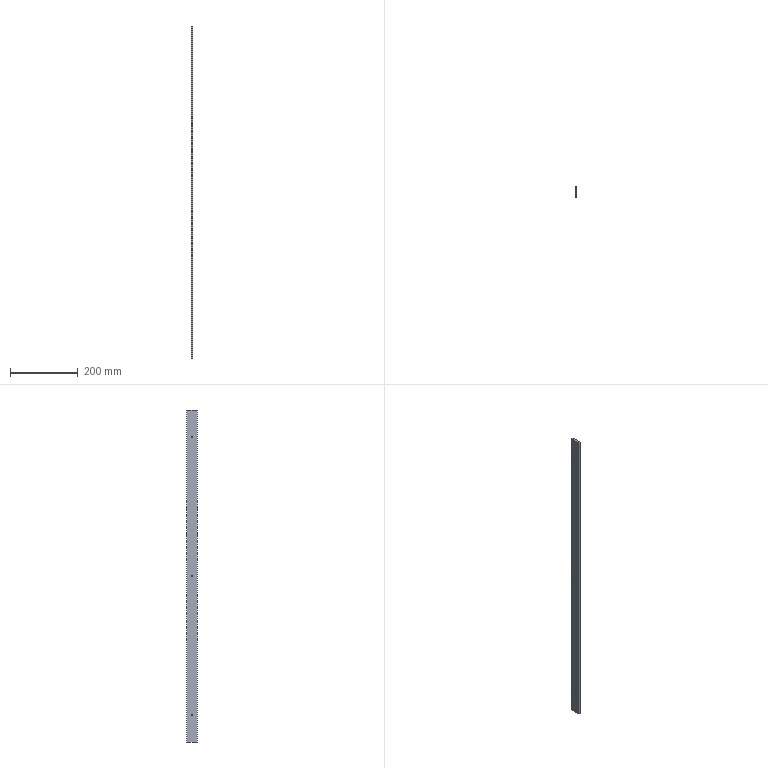Part | NX | features solid 2 | 1 solid | 12 faces | box 5 x 30 x 980 mm | volume 146715 mm3 | cylinder 6 | plane 6 | commonest cylinder face diameters 4.917 x6
STEP:
#1=CARTESIAN_POINT('',(-325.,487.459,347.));
#2=VERTEX_POINT('',#1);
#3=CARTESIAN_POINT('',(-330.,487.459,347.));
#4=VERTEX_POINT('',#3);
#5=CARTESIAN_POINT('',(650.472,487.459,347.));
#6=DIRECTION('',(-1.,0.,0.));
#7=VECTOR('',#6,1000.);
#8=LINE('',#5,#7);
#9=EDGE_CURVE('',#2,#4,#8,.T.);
#10=ORIENTED_EDGE('',*,*,#9,.F.);
#11=CARTESIAN_POINT('',(-325.,482.541,347.));
#12=VERTEX_POINT('',#11);
#13=CARTESIAN_POINT('',(-325.,485.,347.));
#14=DIRECTION('',(1.,0.,0.));
#15=DIRECTION('',(0.,1.,0.));
#16=AXIS2_PLACEMENT_3D('',#13,#14,#15);
#17=CIRCLE('',#16,2.458);
#18=EDGE_CURVE('',#2,#12,#17,.T.);
#19=ORIENTED_EDGE('',*,*,#18,.T.);
#20=CARTESIAN_POINT('',(-330.,482.541,347.));
#21=VERTEX_POINT('',#20);
#22=CARTESIAN_POINT('',(650.472,482.541,347.));
#23=DIRECTION('',(-1.,0.,0.));
#24=VECTOR('',#23,1000.);
#25=LINE('',#22,#24);
#26=EDGE_CURVE('',#21,#12,#25,.F.);
#27=ORIENTED_EDGE('',*,*,#26,.F.);
#28=CARTESIAN_POINT('',(-330.,485.,347.));
#29=DIRECTION('',(-1.,0.,0.));
#30=DIRECTION('',(0.,0.,1.));
#31=AXIS2_PLACEMENT_3D('',#28,#29,#30);
#32=CIRCLE('',#31,2.458);
#33=EDGE_CURVE('',#21,#4,#32,.T.);
#34=ORIENTED_EDGE('',*,*,#33,.T.);
#35=EDGE_LOOP('',(#10,#19,#27,#34));
#36=FACE_BOUND('',#35,.T.);
#37=CARTESIAN_POINT('',(650.472,485.,347.));
#38=DIRECTION('',(-1.,0.,0.));
#39=DIRECTION('',(0.,-1.,0.));
#40=AXIS2_PLACEMENT_3D('',#37,#38,#39);
#41=CYLINDRICAL_SURFACE('',#40,2.458);
#42=ADVANCED_FACE('',(#36),#41,.F.);
#43=CARTESIAN_POINT('',(-325.,487.459,1167.));
#44=VERTEX_POINT('',#43);
#45=CARTESIAN_POINT('',(-330.,487.459,1167.));
#46=VERTEX_POINT('',#45);
#47=CARTESIAN_POINT('',(650.472,487.459,1167.));
#48=DIRECTION('',(-1.,0.,0.));
#49=VECTOR('',#48,1000.);
#50=LINE('',#47,#49);
#51=EDGE_CURVE('',#44,#46,#50,.T.);
#52=ORIENTED_EDGE('',*,*,#51,.F.);
#53=CARTESIAN_POINT('',(-325.,482.541,1167.));
#54=VERTEX_POINT('',#53);
#55=CARTESIAN_POINT('',(-325.,485.,1167.));
#56=DIRECTION('',(1.,0.,0.));
#57=DIRECTION('',(0.,1.,0.));
#58=AXIS2_PLACEMENT_3D('',#55,#56,#57);
#59=CIRCLE('',#58,2.458);
#60=EDGE_CURVE('',#44,#54,#59,.T.);
#61=ORIENTED_EDGE('',*,*,#60,.T.);
#62=CARTESIAN_POINT('',(-330.,482.541,1167.));
#63=VERTEX_POINT('',#62);
#64=CARTESIAN_POINT('',(650.472,482.541,1167.));
#65=DIRECTION('',(-1.,0.,0.));
#66=VECTOR('',#65,1000.);
#67=LINE('',#64,#66);
#68=EDGE_CURVE('',#63,#54,#67,.F.);
#69=ORIENTED_EDGE('',*,*,#68,.F.);
#70=CARTESIAN_POINT('',(-330.,485.,1167.));
#71=DIRECTION('',(-1.,0.,0.));
#72=DIRECTION('',(0.,0.,1.));
#73=AXIS2_PLACEMENT_3D('',#70,#71,#72);
#74=CIRCLE('',#73,2.458);
#75=EDGE_CURVE('',#63,#46,#74,.T.);
#76=ORIENTED_EDGE('',*,*,#75,.T.);
#77=EDGE_LOOP('',(#52,#61,#69,#76));
#78=FACE_BOUND('',#77,.T.);
#79=CARTESIAN_POINT('',(650.472,485.,1167.));
#80=DIRECTION('',(-1.,0.,0.));
#81=DIRECTION('',(0.,-1.,0.));
#82=AXIS2_PLACEMENT_3D('',#79,#80,#81);
#83=CYLINDRICAL_SURFACE('',#82,2.458);
#84=ADVANCED_FACE('',(#78),#83,.F.);
#85=CARTESIAN_POINT('',(-330.,487.459,757.));
#86=VERTEX_POINT('',#85);
#87=CARTESIAN_POINT('',(-325.,487.459,757.));
#88=VERTEX_POINT('',#87);
#89=CARTESIAN_POINT('',(650.472,487.459,757.));
#90=DIRECTION('',(-1.,0.,0.));
#91=VECTOR('',#90,1000.);
#92=LINE('',#89,#91);
#93=EDGE_CURVE('',#86,#88,#92,.F.);
#94=ORIENTED_EDGE('',*,*,#93,.T.);
#95=CARTESIAN_POINT('',(-325.,482.541,757.));
#96=VERTEX_POINT('',#95);
#97=CARTESIAN_POINT('',(-325.,485.,757.));
#98=DIRECTION('',(1.,0.,0.));
#99=DIRECTION('',(0.,1.,0.));
#100=AXIS2_PLACEMENT_3D('',#97,#98,#99);
#101=CIRCLE('',#100,2.458);
#102=EDGE_CURVE('',#88,#96,#101,.T.);
#103=ORIENTED_EDGE('',*,*,#102,.T.);
#104=CARTESIAN_POINT('',(-330.,482.541,757.));
#105=VERTEX_POINT('',#104);
#106=CARTESIAN_POINT('',(650.472,482.541,757.));
#107=DIRECTION('',(-1.,0.,0.));
#108=VECTOR('',#107,1000.);
#109=LINE('',#106,#108);
#110=EDGE_CURVE('',#96,#105,#109,.T.);
#111=ORIENTED_EDGE('',*,*,#110,.T.);
#112=CARTESIAN_POINT('',(-330.,485.,757.));
#113=DIRECTION('',(-1.,0.,0.));
#114=DIRECTION('',(0.,0.,1.));
#115=AXIS2_PLACEMENT_3D('',#112,#113,#114);
#116=CIRCLE('',#115,2.459);
#117=EDGE_CURVE('',#105,#86,#116,.T.);
#118=ORIENTED_EDGE('',*,*,#117,.T.);
#119=EDGE_LOOP('',(#94,#103,#111,#118));
#120=FACE_BOUND('',#119,.T.);
#121=CARTESIAN_POINT('',(650.472,485.,757.));
#122=DIRECTION('',(-1.,0.,0.));
#123=DIRECTION('',(0.,-1.,0.));
#124=AXIS2_PLACEMENT_3D('',#121,#122,#123);
#125=CYLINDRICAL_SURFACE('',#124,2.458);
#126=ADVANCED_FACE('',(#120),#125,.F.);
#127=ORIENTED_EDGE('',*,*,#117,.F.);
#128=CARTESIAN_POINT('',(-330.,485.,757.));
#129=DIRECTION('',(-1.,0.,0.));
#130=DIRECTION('',(0.,0.,1.));
#131=AXIS2_PLACEMENT_3D('',#128,#129,#130);
#132=CIRCLE('',#131,2.459);
#133=EDGE_CURVE('',#86,#105,#132,.T.);
#134=ORIENTED_EDGE('',*,*,#133,.F.);
#135=EDGE_LOOP('',(#127,#134));
#136=FACE_BOUND('',#135,.T.);
#137=ORIENTED_EDGE('',*,*,#75,.F.);
#138=CARTESIAN_POINT('',(-330.,485.,1167.));
#139=DIRECTION('',(-1.,0.,0.));
#140=DIRECTION('',(0.,0.,1.));
#141=AXIS2_PLACEMENT_3D('',#138,#139,#140);
#142=CIRCLE('',#141,2.458);
#143=EDGE_CURVE('',#46,#63,#142,.T.);
#144=ORIENTED_EDGE('',*,*,#143,.F.);
#145=EDGE_LOOP('',(#137,#144));
#146=FACE_BOUND('',#145,.T.);
#147=ORIENTED_EDGE('',*,*,#33,.F.);
#148=CARTESIAN_POINT('',(-330.,485.,347.));
#149=DIRECTION('',(-1.,0.,0.));
#150=DIRECTION('',(0.,0.,1.));
#151=AXIS2_PLACEMENT_3D('',#148,#149,#150);
#152=CIRCLE('',#151,2.458);
#153=EDGE_CURVE('',#4,#21,#152,.T.);
#154=ORIENTED_EDGE('',*,*,#153,.F.);
#155=EDGE_LOOP('',(#147,#154));
#156=FACE_BOUND('',#155,.T.);
#157=CARTESIAN_POINT('',(-330.,470.,267.));
#158=VERTEX_POINT('',#157);
#159=CARTESIAN_POINT('',(-330.,500.,267.));
#160=VERTEX_POINT('',#159);
#161=CARTESIAN_POINT('',(-330.,470.,267.));
#162=DIRECTION('',(0.,1.,0.));
#163=VECTOR('',#162,1000.);
#164=LINE('',#161,#163);
#165=EDGE_CURVE('',#158,#160,#164,.T.);
#166=ORIENTED_EDGE('',*,*,#165,.F.);
#167=CARTESIAN_POINT('',(-330.,470.,1247.));
#168=VERTEX_POINT('',#167);
#169=CARTESIAN_POINT('',(-330.,470.,1247.));
#170=DIRECTION('',(0.,0.,-1.));
#171=VECTOR('',#170,1000.);
#172=LINE('',#169,#171);
#173=EDGE_CURVE('',#168,#158,#172,.T.);
#174=ORIENTED_EDGE('',*,*,#173,.F.);
#175=CARTESIAN_POINT('',(-330.,500.,1247.));
#176=VERTEX_POINT('',#175);
#177=CARTESIAN_POINT('',(-330.,500.,1247.));
#178=DIRECTION('',(0.,-1.,0.));
#179=VECTOR('',#178,1000.);
#180=LINE('',#177,#179);
#181=EDGE_CURVE('',#176,#168,#180,.T.);
#182=ORIENTED_EDGE('',*,*,#181,.F.);
#183=CARTESIAN_POINT('',(-330.,500.,267.));
#184=DIRECTION('',(0.,0.,1.));
#185=VECTOR('',#184,1000.);
#186=LINE('',#183,#185);
#187=EDGE_CURVE('',#160,#176,#186,.T.);
#188=ORIENTED_EDGE('',*,*,#187,.F.);
#189=EDGE_LOOP('',(#166,#174,#182,#188));
#190=FACE_BOUND('',#189,.T.);
#191=CARTESIAN_POINT('',(-330.,485.,757.));
#192=DIRECTION('',(1.,0.,0.));
#193=DIRECTION('',(0.,1.,0.));
#194=AXIS2_PLACEMENT_3D('',#191,#192,#193);
#195=PLANE('',#194);
#196=ADVANCED_FACE('',(#136,#146,#156,#190),#195,.F.);
#197=CARTESIAN_POINT('',(-325.,485.,757.));
#198=DIRECTION('',(1.,0.,0.));
#199=DIRECTION('',(0.,1.,0.));
#200=AXIS2_PLACEMENT_3D('',#197,#198,#199);
#201=CIRCLE('',#200,2.458);
#202=EDGE_CURVE('',#96,#88,#201,.T.);
#203=ORIENTED_EDGE('',*,*,#202,.F.);
#204=ORIENTED_EDGE('',*,*,#102,.F.);
#205=EDGE_LOOP('',(#203,#204));
#206=FACE_BOUND('',#205,.T.);
#207=CARTESIAN_POINT('',(-325.,485.,1167.));
#208=DIRECTION('',(1.,0.,0.));
#209=DIRECTION('',(0.,1.,0.));
#210=AXIS2_PLACEMENT_3D('',#207,#208,#209);
#211=CIRCLE('',#210,2.458);
#212=EDGE_CURVE('',#54,#44,#211,.T.);
#213=ORIENTED_EDGE('',*,*,#212,.F.);
#214=ORIENTED_EDGE('',*,*,#60,.F.);
#215=EDGE_LOOP('',(#213,#214));
#216=FACE_BOUND('',#215,.T.);
#217=CARTESIAN_POINT('',(-325.,485.,347.));
#218=DIRECTION('',(1.,0.,0.));
#219=DIRECTION('',(0.,1.,0.));
#220=AXIS2_PLACEMENT_3D('',#217,#218,#219);
#221=CIRCLE('',#220,2.458);
#222=EDGE_CURVE('',#12,#2,#221,.T.);
#223=ORIENTED_EDGE('',*,*,#222,.F.);
#224=ORIENTED_EDGE('',*,*,#18,.F.);
#225=EDGE_LOOP('',(#223,#224));
#226=FACE_BOUND('',#225,.T.);
#227=CARTESIAN_POINT('',(-325.,470.,267.));
#228=VERTEX_POINT('',#227);
#229=CARTESIAN_POINT('',(-325.,500.,267.));
#230=VERTEX_POINT('',#229);
#231=CARTESIAN_POINT('',(-325.,470.,267.));
#232=DIRECTION('',(0.,1.,0.));
#233=VECTOR('',#232,1000.);
#234=LINE('',#231,#233);
#235=EDGE_CURVE('',#228,#230,#234,.T.);
#236=ORIENTED_EDGE('',*,*,#235,.T.);
#237=CARTESIAN_POINT('',(-325.,500.,1247.));
#238=VERTEX_POINT('',#237);
#239=CARTESIAN_POINT('',(-325.,500.,267.));
#240=DIRECTION('',(0.,0.,1.));
#241=VECTOR('',#240,1000.);
#242=LINE('',#239,#241);
#243=EDGE_CURVE('',#230,#238,#242,.T.);
#244=ORIENTED_EDGE('',*,*,#243,.T.);
#245=CARTESIAN_POINT('',(-325.,470.,1247.));
#246=VERTEX_POINT('',#245);
#247=CARTESIAN_POINT('',(-325.,500.,1247.));
#248=DIRECTION('',(0.,-1.,0.));
#249=VECTOR('',#248,1000.);
#250=LINE('',#247,#249);
#251=EDGE_CURVE('',#238,#246,#250,.T.);
#252=ORIENTED_EDGE('',*,*,#251,.T.);
#253=CARTESIAN_POINT('',(-325.,470.,1247.));
#254=DIRECTION('',(0.,0.,-1.));
#255=VECTOR('',#254,1000.);
#256=LINE('',#253,#255);
#257=EDGE_CURVE('',#246,#228,#256,.T.);
#258=ORIENTED_EDGE('',*,*,#257,.T.);
#259=EDGE_LOOP('',(#236,#244,#252,#258));
#260=FACE_BOUND('',#259,.T.);
#261=CARTESIAN_POINT('',(-325.,485.,757.));
#262=DIRECTION('',(1.,0.,0.));
#263=DIRECTION('',(0.,1.,0.));
#264=AXIS2_PLACEMENT_3D('',#261,#262,#263);
#265=PLANE('',#264);
#266=ADVANCED_FACE('',(#206,#216,#226,#260),#265,.T.);
#267=ORIENTED_EDGE('',*,*,#173,.T.);
#268=CARTESIAN_POINT('',(-325.,470.,267.));
#269=DIRECTION('',(-1.,0.,0.));
#270=VECTOR('',#269,1000.);
#271=LINE('',#268,#270);
#272=EDGE_CURVE('',#228,#158,#271,.T.);
#273=ORIENTED_EDGE('',*,*,#272,.F.);
#274=ORIENTED_EDGE('',*,*,#257,.F.);
#275=CARTESIAN_POINT('',(-325.,470.,1247.));
#276=DIRECTION('',(-1.,0.,0.));
#277=VECTOR('',#276,1000.);
#278=LINE('',#275,#277);
#279=EDGE_CURVE('',#246,#168,#278,.T.);
#280=ORIENTED_EDGE('',*,*,#279,.T.);
#281=EDGE_LOOP('',(#267,#273,#274,#280));
#282=FACE_BOUND('',#281,.T.);
#283=CARTESIAN_POINT('',(-325.,470.,1247.));
#284=DIRECTION('',(0.,1.,0.));
#285=DIRECTION('',(1.,0.,0.));
#286=AXIS2_PLACEMENT_3D('',#283,#284,#285);
#287=PLANE('',#286);
#288=ADVANCED_FACE('',(#282),#287,.F.);
#289=ORIENTED_EDGE('',*,*,#181,.T.);
#290=ORIENTED_EDGE('',*,*,#279,.F.);
#291=ORIENTED_EDGE('',*,*,#251,.F.);
#292=CARTESIAN_POINT('',(-325.,500.,1247.));
#293=DIRECTION('',(-1.,0.,0.));
#294=VECTOR('',#293,1000.);
#295=LINE('',#292,#294);
#296=EDGE_CURVE('',#238,#176,#295,.T.);
#297=ORIENTED_EDGE('',*,*,#296,.T.);
#298=EDGE_LOOP('',(#289,#290,#291,#297));
#299=FACE_BOUND('',#298,.T.);
#300=CARTESIAN_POINT('',(-325.,500.,1247.));
#301=DIRECTION('',(0.,0.,-1.));
#302=DIRECTION('',(0.,-1.,0.));
#303=AXIS2_PLACEMENT_3D('',#300,#301,#302);
#304=PLANE('',#303);
#305=ADVANCED_FACE('',(#299),#304,.F.);
#306=ORIENTED_EDGE('',*,*,#187,.T.);
#307=ORIENTED_EDGE('',*,*,#296,.F.);
#308=ORIENTED_EDGE('',*,*,#243,.F.);
#309=CARTESIAN_POINT('',(-325.,500.,267.));
#310=DIRECTION('',(-1.,0.,0.));
#311=VECTOR('',#310,1000.);
#312=LINE('',#309,#311);
#313=EDGE_CURVE('',#230,#160,#312,.T.);
#314=ORIENTED_EDGE('',*,*,#313,.T.);
#315=EDGE_LOOP('',(#306,#307,#308,#314));
#316=FACE_BOUND('',#315,.T.);
#317=CARTESIAN_POINT('',(-325.,500.,267.));
#318=DIRECTION('',(0.,-1.,0.));
#319=DIRECTION('',(0.,0.,-1.));
#320=AXIS2_PLACEMENT_3D('',#317,#318,#319);
#321=PLANE('',#320);
#322=ADVANCED_FACE('',(#316),#321,.F.);
#323=ORIENTED_EDGE('',*,*,#165,.T.);
#324=ORIENTED_EDGE('',*,*,#313,.F.);
#325=ORIENTED_EDGE('',*,*,#235,.F.);
#326=ORIENTED_EDGE('',*,*,#272,.T.);
#327=EDGE_LOOP('',(#323,#324,#325,#326));
#328=FACE_BOUND('',#327,.T.);
#329=CARTESIAN_POINT('',(-325.,470.,267.));
#330=DIRECTION('',(0.,0.,1.));
#331=DIRECTION('',(1.,0.,0.));
#332=AXIS2_PLACEMENT_3D('',#329,#330,#331);
#333=PLANE('',#332);
#334=ADVANCED_FACE('',(#328),#333,.F.);
#335=ORIENTED_EDGE('',*,*,#202,.T.);
#336=ORIENTED_EDGE('',*,*,#93,.F.);
#337=ORIENTED_EDGE('',*,*,#133,.T.);
#338=ORIENTED_EDGE('',*,*,#110,.F.);
#339=EDGE_LOOP('',(#335,#336,#337,#338));
#340=FACE_BOUND('',#339,.T.);
#341=CARTESIAN_POINT('',(650.472,485.,757.));
#342=DIRECTION('',(-1.,0.,0.));
#343=DIRECTION('',(0.,-1.,0.));
#344=AXIS2_PLACEMENT_3D('',#341,#342,#343);
#345=CYLINDRICAL_SURFACE('',#344,2.458);
#346=ADVANCED_FACE('',(#340),#345,.F.);
#347=ORIENTED_EDGE('',*,*,#212,.T.);
#348=ORIENTED_EDGE('',*,*,#51,.T.);
#349=ORIENTED_EDGE('',*,*,#143,.T.);
#350=ORIENTED_EDGE('',*,*,#68,.T.);
#351=EDGE_LOOP('',(#347,#348,#349,#350));
#352=FACE_BOUND('',#351,.T.);
#353=CARTESIAN_POINT('',(650.472,485.,1167.));
#354=DIRECTION('',(-1.,0.,0.));
#355=DIRECTION('',(0.,-1.,0.));
#356=AXIS2_PLACEMENT_3D('',#353,#354,#355);
#357=CYLINDRICAL_SURFACE('',#356,2.458);
#358=ADVANCED_FACE('',(#352),#357,.F.);
#359=ORIENTED_EDGE('',*,*,#222,.T.);
#360=ORIENTED_EDGE('',*,*,#9,.T.);
#361=ORIENTED_EDGE('',*,*,#153,.T.);
#362=ORIENTED_EDGE('',*,*,#26,.T.);
#363=EDGE_LOOP('',(#359,#360,#361,#362));
#364=FACE_BOUND('',#363,.T.);
#365=CARTESIAN_POINT('',(650.472,485.,347.));
#366=DIRECTION('',(-1.,0.,0.));
#367=DIRECTION('',(0.,-1.,0.));
#368=AXIS2_PLACEMENT_3D('',#365,#366,#367);
#369=CYLINDRICAL_SURFACE('',#368,2.458);
#370=ADVANCED_FACE('',(#364),#369,.F.);
#371=CLOSED_SHELL('',(#42,#84,#126,#196,#266,#288,#305,#322,#334,#346,#358,#370));
#372=MANIFOLD_SOLID_BREP('',#371);
#373=(LENGTH_UNIT()NAMED_UNIT(*)SI_UNIT(.MILLI.,.METRE.));
#374=UNCERTAINTY_MEASURE_WITH_UNIT(LENGTH_MEASURE(0.00001),#373,'','');
#375=(NAMED_UNIT(*)PLANE_ANGLE_UNIT()SI_UNIT($,.RADIAN.));
#376=(NAMED_UNIT(*)SI_UNIT($,.STERADIAN.)SOLID_ANGLE_UNIT());
#377=(GEOMETRIC_REPRESENTATION_CONTEXT(3)GLOBAL_UNCERTAINTY_ASSIGNED_CONTEXT((#374))GLOBAL_UNIT_ASSIGNED_CONTEXT((#373,#375,#376))REPRESENTATION_CONTEXT('',''));
#378=ADVANCED_BREP_SHAPE_REPRESENTATION('',(#372),#377);